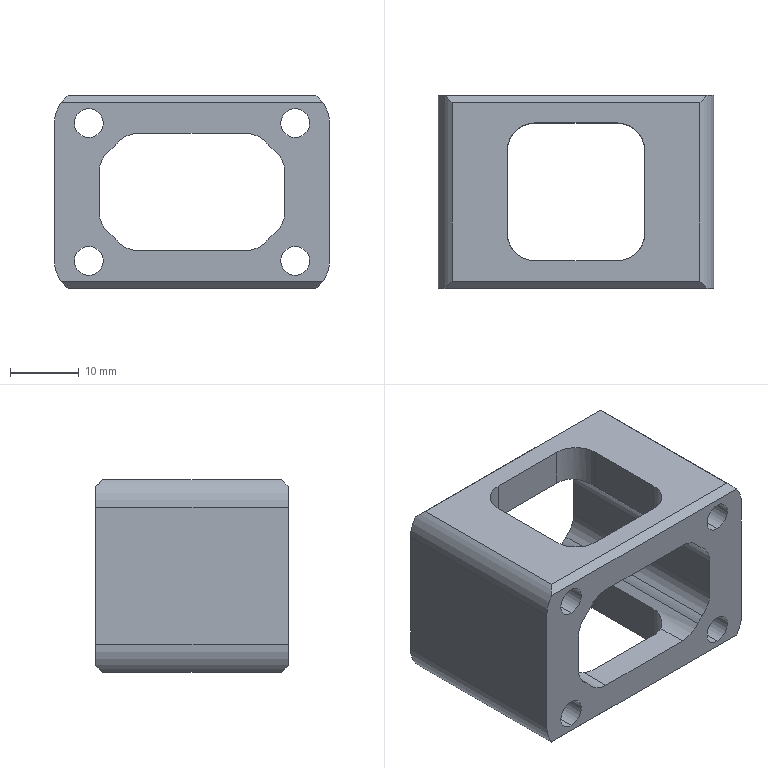Part | SolidWorks | features ICE 3, Fillet 2, Chamfer 1, Extrusion 1 | 1 solid | 56 faces | box 40 x 28 x 28 mm | volume 13306 mm3 | cylinder 32 | plane 24 | commonest cylinder face diameters 8 x16 4.2 x8 10 x8